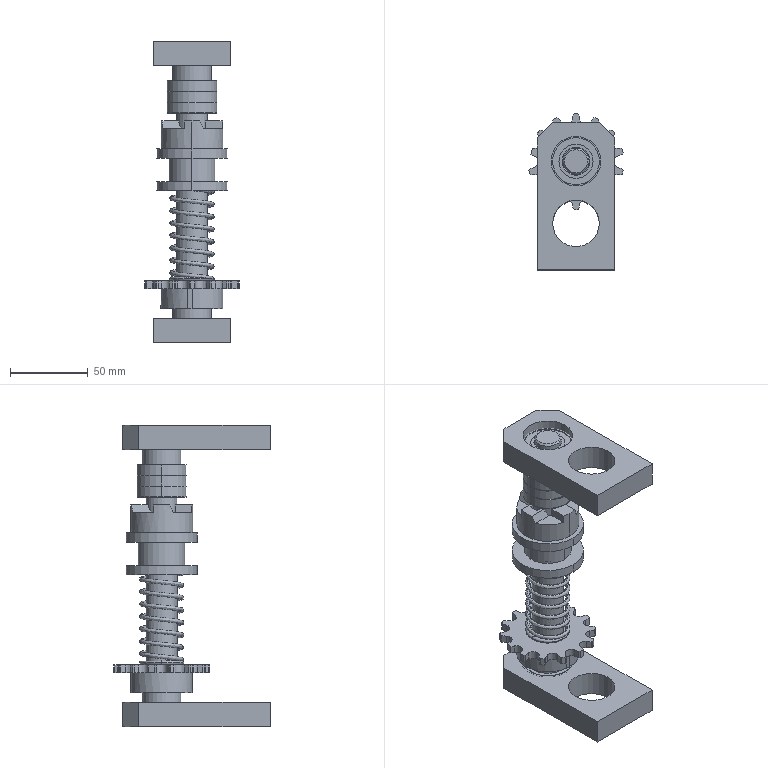Part | NX | features EXTRUDE 9, DATUM_CSYS 7, EXTRACT_DATUM_PLANE 7, SKETCH 7, BREP 4, UNITE 2, CHAMFER 1, Delete Body 1 | 13 solids | 319 faces | box 60.843 x 100.95 x 194.5 mm | volume 245007 mm3 | plane 138 | cylinder 113 | torus 48 | spline 18 | cone 2 | commonest cylinder face diameters 7.77 x14 61.9 x13 20 x12 23.732 x12 28.634 x12 22.033 x8